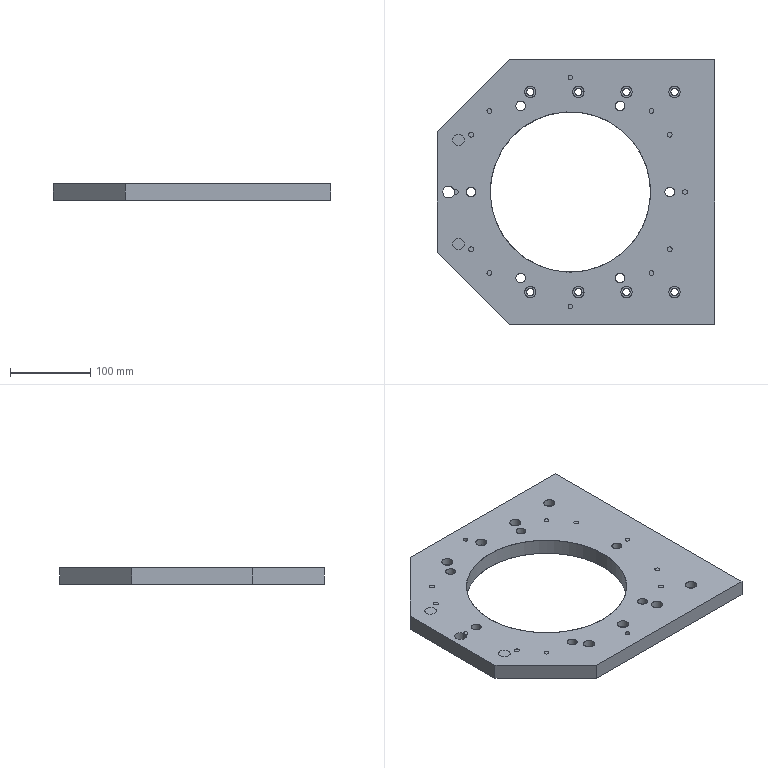NC program | NX | posted with a generic post | part box 346 x 330 x 20 mm
Lines 27998 to 28317 of 28317:
(ZLEVEL_PROFILE_COPY , TOOL : D10JING)
N55952 T09 M6
N55954 G54
N55956 G17 G0 G90 X-168.167 Y182.485 S5000 M3
N55958 G43 Z70. H9
N55960 Z-17.
N55962 G94 G1 Z-20. F1200.
N55964 X-165.866 Y178.5
N55966 G3 X-165. Y178. R1.
N55968 G1 X165.
N55970 G3 X165.866 Y178.5 R1.
N55972 G1 X168.167 Y182.485
N55974 Z-17.
N55976 G0 Z70.
N55978 X78.167 Y-182.485
N55980 Z-17.
N55982 G1 Z-20.
N55984 X75.866 Y-178.5
N55986 G3 X75. Y-178. R1.
N55988 G1 X-75.
N55990 G3 X-75.866 Y-178.5 R1.
N55992 G1 X-78.167 Y-182.485
N55994 Z-17.
N55996 G0 Z70.
N55998 M5
(ZLEVEL_PROFILE_COPY_COPY_1 , TOOL : D6)
N56000 T06 M6
N56002 G54
N56004 G17 G0 G90 X-0.262 Y-103.94 S5000 M3
N56006 G43 Z70. H6
N56008 Z-6.95
N56010 G94 G1 Z-9.95 F1200.
N56012 G3 X0. Y-104. R0.6
N56014 X97. Y-7. R97.
N56016 X0. Y-104. R-97.
N56018 X0.262 Y-103.94 R0.6
N56020 G1 Z-6.95
N56022 G0 X-0.262 Z-16.9
N56024 G1 Z-19.9
N56026 G3 X0. Y-104. R0.6
N56028 X97. Y-7. R97.
N56030 X0. Y-104. R-97.
N56032 X0.262 Y-103.94 R0.6
N56034 G1 Z-16.9
N56036 G0 Z70.
N56038 M5
(ZLEVEL_PROFILE_COPY_COPY , TOOL : D6A45)
N56040 T07 M6
N56042 G54
N56044 G17 G0 G90 X1.138 Y120.712 S7500 M3
N56046 G43 Z70. H7
N56048 Z2.
N56050 G94 G1 Z-1. F1200.
N56052 X0.52 Y121.783
N56054 G3 X0. Y122.083 R0.6
N56056 X-5.083 Y117. R5.083
N56058 X0. Y122.083 R-5.083
N56060 X-0.52 Y121.783 R0.6
N56062 G1 X-1.138 Y120.712
N56064 Z2.
N56066 G0 Z70.
N56068 Y-134.712
N56070 Z2.
N56072 G1 Z-1.
N56074 X-0.52 Y-135.783
N56076 G3 X0. Y-136.083 R0.6
N56078 X5.083 Y-131. R5.083
N56080 X0. Y-136.083 R-5.083
N56082 X0.52 Y-135.783 R0.6
N56084 G1 X1.138 Y-134.712
N56086 Z2.
N56088 G0 Z70.
N56090 X-129.754 Y-55.886
N56092 Z2.
N56094 G1 Z-1.
N56096 X-130.783 Y-56.48
N56098 G3 X-131.083 Y-57. R0.6
N56100 X-125. Y-63.083 R6.083
N56102 X-131.083 Y-57. R-6.083
N56104 X-130.783 Y-57.52 R0.6
N56106 G1 X-129.754 Y-58.114
N56108 Z2.
N56110 G0 Z70.
N56112 X-1.109 Y-164.012
N56114 Z2.
N56116 G1 Z-1.
N56118 X-0.52 Y-165.033
N56120 G3 X0. Y-165.333 R0.6
N56122 X6.333 Y-159. R6.333
N56124 X0. Y-165.333 R-6.333
N56126 X0.52 Y-165.033 R0.6
N56128 G1 X1.109 Y-164.012
N56130 Z2.
N56132 G0 Z70.
N56134 X-143.848 Y-6.753
N56136 Z2.
N56138 G1 Z-1.
N56140 X-144.783 Y-6.48
N56142 G3 X-145.083 Y-7. R0.6
N56144 X-143. Y-9.083 R2.083
N56146 X-145.083 Y-7. R-2.083
N56148 X-144.783 Y-7.52 R0.6
N56150 G1 X-143.848 Y-7.247
N56152 Z2.
N56154 G0 Z70.
N56156 X-97.877 Y-5.958
N56158 Z2.
N56160 G1 Z-1.
N56162 X-98.783 Y-6.48
N56164 G3 X-99.083 Y-7. R0.6
N56166 X0. Y-106.083 R99.083
N56168 X-99.083 Y-7. R-99.083
N56170 X-98.783 Y-7.52 R0.6
N56172 G1 X-97.877 Y-8.042
N56174 Z2.
N56176 G0 Z70.
N56178 X71.747 Y117.689
N56180 Z2.
N56182 G1 Z-1.
N56184 X72.02 Y118.624
N56186 G3 X71.5 Y118.924 R0.6
N56188 X69.417 Y116.842 R2.083
N56190 X71.5 Y118.924 R-2.083
N56192 X70.98 Y118.624 R0.6
N56194 G1 X71.253 Y117.689
N56196 Z2.
N56198 G0 Z70.
N56200 Y-131.689
N56202 Z2.
N56204 G1 Z-1.
N56206 X70.98 Y-132.624
N56208 G3 X71.5 Y-132.924 R0.6
N56210 X73.583 Y-130.842 R2.083
N56212 X71.5 Y-132.924 R-2.083
N56214 X72.02 Y-132.624 R0.6
N56216 G1 X71.747 Y-131.689
N56218 Z2.
N56220 G0 Z70.
N56222 X-129.754 Y124.114
N56224 Z2.
N56226 G1 Z-1.
N56228 X-130.783 Y123.52
N56230 G3 X-131.083 Y123. R0.6
N56232 X-125. Y116.917 R6.083
N56234 X-131.083 Y123. R-6.083
N56236 X-130.783 Y122.48 R0.6
N56238 G1 X-129.754 Y121.886
N56240 Z2.
N56242 G0 Z70.
N56244 X-111.1 Y56.138
N56246 Z2.
N56248 G1 Z-1.
N56250 X-112.17 Y55.52
N56252 G3 X-112.47 Y55. R0.6
N56254 X-107.387 Y49.917 R5.083
N56256 X-112.47 Y55. R-5.083
N56258 X-112.17 Y54.48 R0.6
N56260 G1 X-111.1 Y53.862
N56262 Z2.
N56264 G0 Z70.
N56266 X111.1
N56268 Z2.
N56270 G1 Z-1.
N56272 X112.17 Y54.48
N56274 G3 X112.47 Y55. R0.6
N56276 X107.387 Y60.083 R5.083
N56278 X112.47 Y55. R-5.083
N56280 X112.17 Y55.52 R0.6
N56282 G1 X111.1 Y56.138
N56284 Z2.
N56286 G0 Z70.
N56288 Y-70.138
N56290 Z2.
N56292 G1 Z-1.
N56294 X112.17 Y-69.52
N56296 G3 X112.47 Y-69. R0.6
N56298 X107.387 Y-63.917 R5.083
N56300 X112.47 Y-69. R-5.083
N56302 X112.17 Y-68.48 R0.6
N56304 G1 X111.1 Y-67.862
N56306 Z2.
N56308 G0 Z70.
N56310 X-111.1
N56312 Z2.
N56314 G1 Z-1.
N56316 X-112.17 Y-68.48
N56318 G3 X-112.47 Y-69. R0.6
N56320 X-107.387 Y-74.083 R5.083
N56322 X-112.47 Y-69. R-5.083
N56324 X-112.17 Y-69.52 R0.6
N56326 G1 X-111.1 Y-70.138
N56328 Z2.
N56330 G0 Z70.
N56332 X-71.253 Y117.689
N56334 Z2.
N56336 G1 Z-1.
N56338 X-70.98 Y118.624
N56340 G3 X-71.5 Y118.924 R0.6
N56342 X-73.583 Y116.842 R2.083
N56344 X-71.5 Y118.924 R-2.083
N56346 X-72.02 Y118.624 R0.6
N56348 G1 X-71.747 Y117.689
N56350 Z2.
N56352 G0 Z70.
N56354 Y-131.689
N56356 Z2.
N56358 G1 Z-1.
N56360 X-72.02 Y-132.624
N56362 G3 X-71.5 Y-132.924 R0.6
N56364 X-69.417 Y-130.842 R2.083
N56366 X-71.5 Y-132.924 R-2.083
N56368 X-70.98 Y-132.624 R0.6
N56370 G1 X-71.253 Y-131.689
N56372 Z2.
N56374 G0 Z70.
N56376 X-129.754 Y64.114
N56378 Z2.
N56380 G1 Z-1.
N56382 X-130.783 Y63.52
N56384 G3 X-131.083 Y63. R0.6
N56386 X-125. Y56.917 R6.083
N56388 X-131.083 Y63. R-6.083
N56390 X-130.783 Y62.48 R0.6
N56392 G1 X-129.754 Y61.886
N56394 Z2.
N56396 G0 Z70.
N56398 X129.754 Y121.886
N56400 Z2.
N56402 G1 Z-1.
N56404 X130.783 Y122.48
N56406 G3 X131.083 Y123. R0.6
N56408 X125. Y129.083 R6.083
N56410 X131.083 Y123. R-6.083
N56412 X130.783 Y123.52 R0.6
N56414 G1 X129.754 Y124.114
N56416 Z2.
N56418 G0 Z70.
N56420 Y61.886
N56422 Z2.
N56424 G1 Z-1.
N56426 X130.783 Y62.48
N56428 G3 X131.083 Y63. R0.6
N56430 X125. Y69.083 R6.083
N56432 X131.083 Y63. R-6.083
N56434 X130.783 Y63.52 R0.6
N56436 G1 X129.754 Y64.114
N56438 Z2.
N56440 G0 Z70.
N56442 Y1.886
N56444 Z2.
N56446 G1 Z-1.
N56448 X130.783 Y2.48
N56450 G3 X131.083 Y3. R0.6
N56452 X125. Y9.083 R6.083
N56454 X131.083 Y3. R-6.083
N56456 X130.783 Y3.52 R0.6
N56458 G1 X129.754 Y4.114
N56460 Z2.
N56462 G0 Z70.
N56464 Y-58.114
N56466 Z2.
N56468 G1 Z-1.
N56470 X130.783 Y-57.52
N56472 G3 X131.083 Y-57. R0.6
N56474 X125. Y-50.917 R6.083
N56476 X131.083 Y-57. R-6.083
N56478 X130.783 Y-56.48 R0.6
N56480 G1 X129.754 Y-55.886
N56482 Z2.
N56484 G0 Z70.
N56486 X143.848 Y-7.247
N56488 Z2.
N56490 G1 Z-1.
N56492 X144.783 Y-7.52
N56494 G3 X145.083 Y-7. R0.6
N56496 X143. Y-4.917 R2.083
N56498 X145.083 Y-7. R-2.083
N56500 X144.783 Y-6.48 R0.6
N56502 G1 X143.848 Y-6.753
N56504 Z2.
N56506 G0 Z70.
N56508 X-129.754 Y4.114
N56510 Z2.
N56512 G1 Z-1.
N56514 X-130.783 Y3.52
N56516 G3 X-131.083 Y3. R0.6
N56518 X-125. Y-3.083 R6.083
N56520 X-131.083 Y3. R-6.083
N56522 X-130.783 Y2.48 R0.6
N56524 G1 X-129.754 Y1.886
N56526 Z2.
N56528 G0 Z70.
N56530 X-165.073 Y175.195
N56532 Z2.
N56534 G1 Z-1.
N56536 X-164.973 Y174.396
N56538 G3 X-164.611 Y173.917 R0.6
N56540 G1 X164.596
N56542 G3 X164.95 Y174.401 R0.6
N56544 G1 X165.037 Y175.202
N56546 Z2.
N56548 G0 Z70.
N56550 X75.069 Y-175.196
N56552 Z2.
N56554 G1 Z-1.
N56556 X74.972 Y-174.397
N56558 G3 X74.611 Y-173.917 R0.6
N56560 G1 X-74.611
N56562 G3 X-74.972 Y-174.397 R0.6
N56564 G1 X-75.069 Y-175.196
N56566 Z2.
N56568 G0 Z70.
N56570 M5
N56572 M2